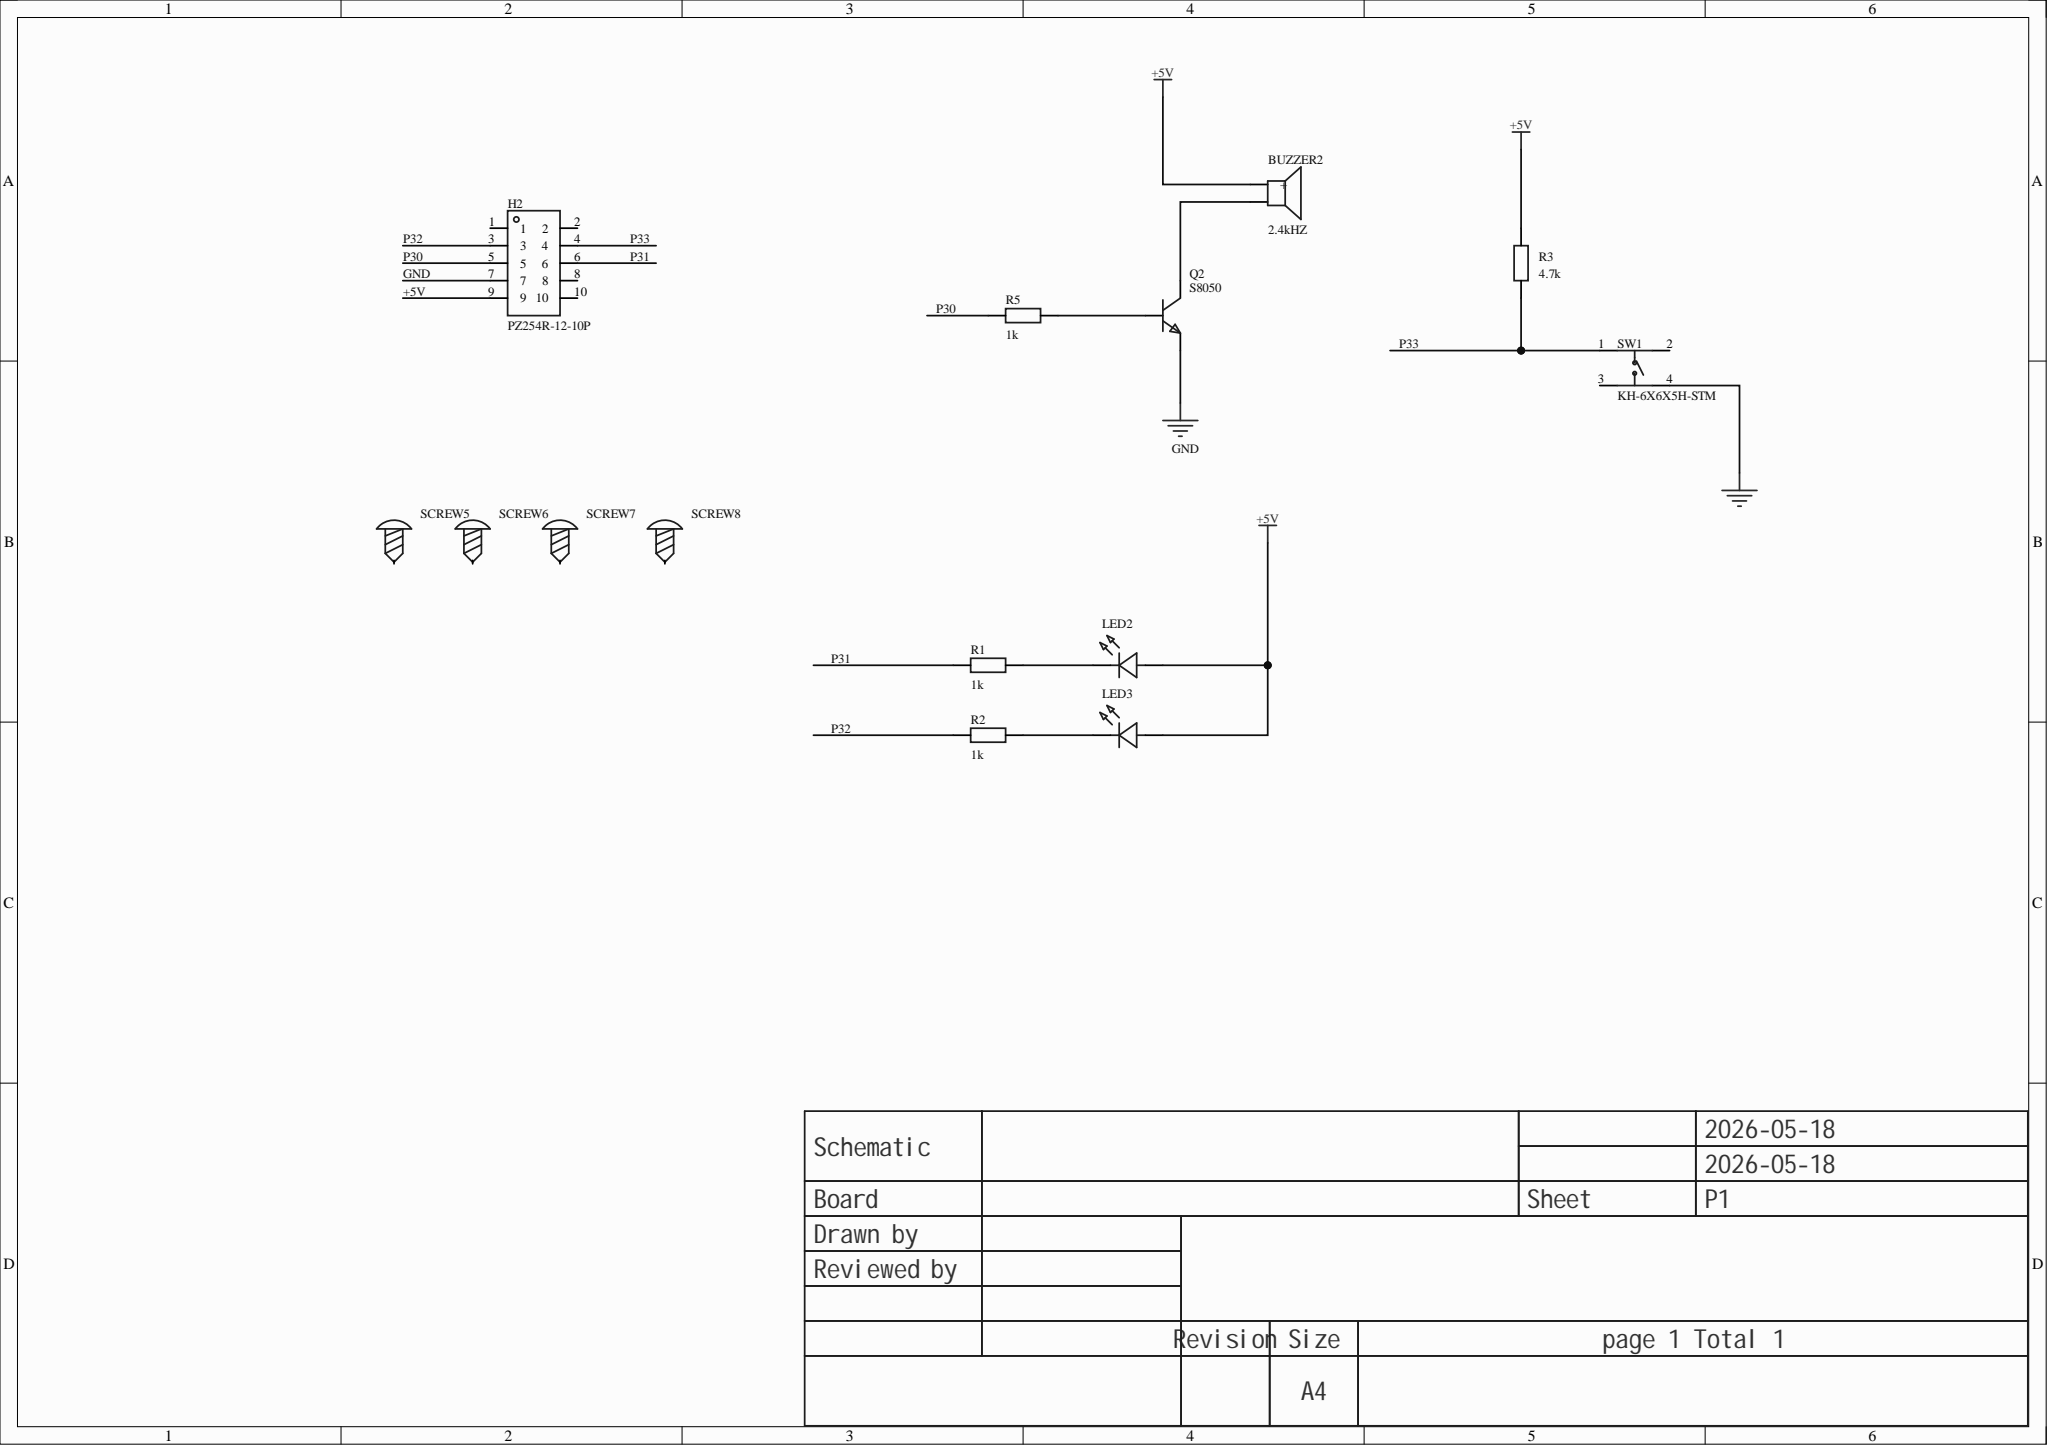Circuit board | Altium Designer | 14 parts | 7 nets
Bill of materials:
Comment,Description,Designator,Footprint,LibRef,Quantity
"2.4kHZ","Drive mode: active (built-in driver circuit); construction: electromagnetic; rated voltage: 5V; operating voltage: 4V~8V; frequency: 2300Hz; sound pressure (SPL): 85dB@5V,10cm; diameter (fD): 12mm; height: 9.8mm;","BUZZER2","BUZ-TH_BD12.0-P7.60-D0.6-FD","TMB12A05_C96093","1"
"PZ254R-12-10P","Pin structure: 2x5P; pitch: 2.54mm; row spacing: 2.54mm; round/square pin: square pin; mounting: right-angle; rows: dual row; total pins: 10P; rated current: -; rated voltage: -; mating pin length: 6mm; insulation height: 2.5mm; contact material: brass; contact plating: -; operating temperature: -40℃~+105℃; color: black;","H2","HDR-TH_10P-P2.54-H-M-R2-C5-S2.54","PZ254R-12-10P","1"
"GL0805UR01","Lamp holder type: 2mmx1.25mm square lamp holder; illumination color: red; forward voltage (Vf): 2.1V; power: -; forward current: 20mA; wavelength: 618nm~624nm; diode configuration: independent diode; lens color: clear lens; color temperature: -; luminous intensity: 100mcd; viewing angle: 120°; mounting: surface mount; operating temperature: -40℃~+85℃;","LED2, LED3","LED0805-R-RD_RED","GL0805UR01","2"
"S8050","Transistor type: NPN; collector current (Ic): 500mA; collector-emitter breakdown voltage (Vceo): 25V; power dissipation (Pd): 300mW; DC current gain (hFE): 120@50mA,1.0V;","Q2","SOT-23-3_L2.9-W1.3-P1.90-LS2.3-BR","S8050_C20069125","1"
"1k","","R1, R2, R5","R0805","Res_0805","3"
"4.7k","","R3","R0805","Res_0805","1"
"","","SCREW5, SCREW6, SCREW7, SCREW8","M3螺丝","M3螺丝","4"
"KH-6X6X5H-STM","Circuit: SPDT; Button shape: round; Mounting: upright SMD; Length: 6mm; Width: 6mm; Height: 5mm; Bracket: none; Contact current: 50mA; Rated voltage: 12V; Life: 8万 cycles;","SW1","SW-SMD_4P-L6.0-W6.0-P4.50-LS9.0_H5.0","KH-6X6X5H-STM","1"
Netlist (Protel format):
[
BUZZER2
BUZ-TH_BD12.0-P7.60-D0.6-FD
2.4kHZ



]
[
H2
HDR-TH_10P-P2.54-H-M-R2-C5-S2.54
PZ254R-12-10P



]
[
LED2
LED0805-R-RD_RED
GL0805UR01



]
[
LED3
LED0805-R-RD_RED
GL0805UR01



]
[
Q2
SOT-23-3_L2.9-W1.3-P1.90-LS2.3-BR
S8050



]
[
R1
R0805
1k



]
[
R2
R0805
1k



]
[
R3
R0805
4.7k



]
[
R5
R0805
1k



]
[
SCREW5
M3螺丝




]
[
SCREW6
M3螺丝




]
[
SCREW7
M3螺丝




]
[
SCREW8
M3螺丝




]
[
SW1
SW-SMD_4P-L6.0-W6.0-P4.50-LS9.0_H5.0
KH-6X6X5H-STM



]
(
NetR3_1
R3-1
SW1-1
)
(
NetQ2_1
Q2-1
R5-2
)
(
NetLED3_2
LED3-2
R2-2
)
(
NetLED2_2
LED2-2
R1-2
)
(
NetBUZZER2_2
BUZZER2-2
Q2-3
)
(
GND
Q2-2
SW1-4
)
(
+5V
BUZZER2-1
LED2-1
LED3-1
R3-2
)